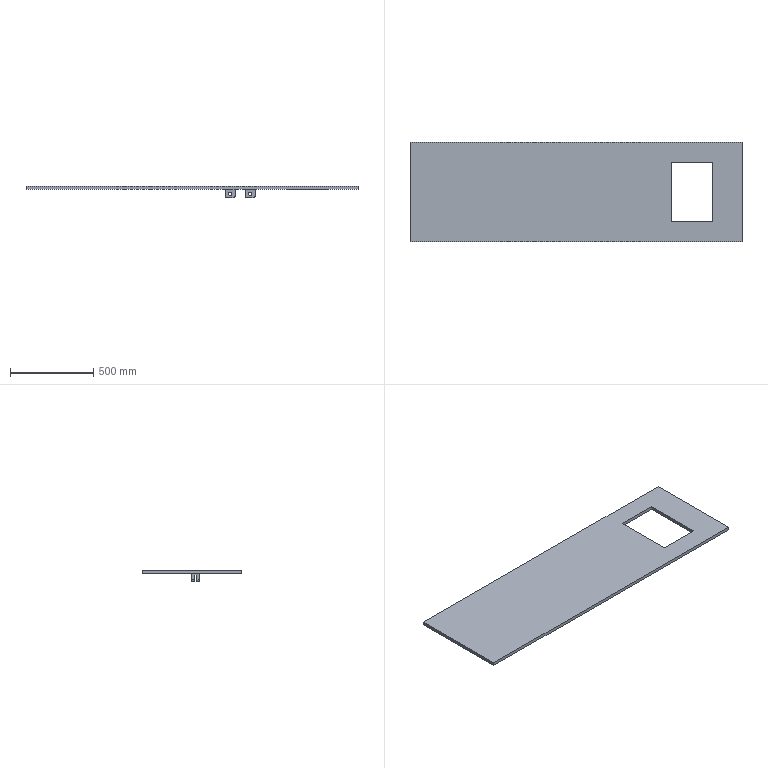Part | SolidWorks | features ICE 3, Cut 1, Extrusion 1, Fillet 1, LPattern 1 | 1 solid | 44 faces | box 2000 x 600 x 71 mm | volume 22419827 mm3 | plane 28 | cylinder 16 | commonest cylinder face diameters 20 x8 24 x8
STEP:
#1=CARTESIAN_POINT('',(220.,2.5,-26.));
#2=VERTEX_POINT('',#1);
#3=CARTESIAN_POINT('',(240.,2.5,-26.));
#4=VERTEX_POINT('',#3);
#5=CARTESIAN_POINT('',(230.,2.5,-26.));
#6=DIRECTION('',(0.,-1.,0.));
#7=DIRECTION('',(1.,0.,0.));
#8=AXIS2_PLACEMENT_3D('',#5,#6,#7);
#9=CIRCLE('',#8,10.);
#10=EDGE_CURVE('',#2,#4,#9,.T.);
#11=ORIENTED_EDGE('',*,*,#10,.F.);
#12=CARTESIAN_POINT('',(220.,-17.5,-26.));
#13=VERTEX_POINT('',#12);
#14=CARTESIAN_POINT('',(220.,300.,-26.));
#15=DIRECTION('',(0.,-1.,0.));
#16=VECTOR('',#15,1000.);
#17=LINE('',#14,#16);
#18=EDGE_CURVE('',#2,#13,#17,.T.);
#19=ORIENTED_EDGE('',*,*,#18,.T.);
#20=CARTESIAN_POINT('',(240.,-17.5,-26.));
#21=VERTEX_POINT('',#20);
#22=CARTESIAN_POINT('',(230.,-17.5,-26.));
#23=DIRECTION('',(0.,1.,0.));
#24=DIRECTION('',(0.,0.,1.));
#25=AXIS2_PLACEMENT_3D('',#22,#23,#24);
#26=CIRCLE('',#25,10.);
#27=EDGE_CURVE('',#21,#13,#26,.T.);
#28=ORIENTED_EDGE('',*,*,#27,.F.);
#29=CARTESIAN_POINT('',(240.,300.,-26.));
#30=DIRECTION('',(0.,-1.,0.));
#31=VECTOR('',#30,1000.);
#32=LINE('',#29,#31);
#33=EDGE_CURVE('',#4,#21,#32,.T.);
#34=ORIENTED_EDGE('',*,*,#33,.F.);
#35=EDGE_LOOP('',(#11,#19,#28,#34));
#36=FACE_OUTER_BOUND('',#35,.T.);
#37=CARTESIAN_POINT('',(230.,300.,-26.));
#38=DIRECTION('',(0.,-1.,0.));
#39=DIRECTION('',(1.,0.,0.));
#40=AXIS2_PLACEMENT_3D('',#37,#38,#39);
#41=CYLINDRICAL_SURFACE('',#40,10.);
#42=ADVANCED_FACE('',(#36),#41,.F.);
#43=CARTESIAN_POINT('',(220.,-29.5,-26.));
#44=VERTEX_POINT('',#43);
#45=CARTESIAN_POINT('',(240.,-29.5,-26.));
#46=VERTEX_POINT('',#45);
#47=CARTESIAN_POINT('',(230.,-29.5,-26.));
#48=DIRECTION('',(0.,-1.,0.));
#49=DIRECTION('',(0.,0.,-1.));
#50=AXIS2_PLACEMENT_3D('',#47,#48,#49);
#51=CIRCLE('',#50,10.);
#52=EDGE_CURVE('',#44,#46,#51,.T.);
#53=ORIENTED_EDGE('',*,*,#52,.F.);
#54=CARTESIAN_POINT('',(220.,-47.5,-26.));
#55=VERTEX_POINT('',#54);
#56=CARTESIAN_POINT('',(220.,300.,-26.));
#57=DIRECTION('',(0.,-1.,0.));
#58=VECTOR('',#57,1000.);
#59=LINE('',#56,#58);
#60=EDGE_CURVE('',#44,#55,#59,.T.);
#61=ORIENTED_EDGE('',*,*,#60,.T.);
#62=CARTESIAN_POINT('',(240.,-47.5,-26.));
#63=VERTEX_POINT('',#62);
#64=CARTESIAN_POINT('',(230.,-47.5,-26.));
#65=DIRECTION('',(0.,-1.,0.));
#66=DIRECTION('',(1.,0.,0.));
#67=AXIS2_PLACEMENT_3D('',#64,#65,#66);
#68=CIRCLE('',#67,10.);
#69=EDGE_CURVE('',#55,#63,#68,.T.);
#70=ORIENTED_EDGE('',*,*,#69,.T.);
#71=CARTESIAN_POINT('',(240.,300.,-26.));
#72=DIRECTION('',(0.,-1.,0.));
#73=VECTOR('',#72,1000.);
#74=LINE('',#71,#73);
#75=EDGE_CURVE('',#46,#63,#74,.T.);
#76=ORIENTED_EDGE('',*,*,#75,.F.);
#77=EDGE_LOOP('',(#53,#61,#70,#76));
#78=FACE_OUTER_BOUND('',#77,.T.);
#79=CARTESIAN_POINT('',(230.,300.,-26.));
#80=DIRECTION('',(0.,-1.,0.));
#81=DIRECTION('',(1.,0.,0.));
#82=AXIS2_PLACEMENT_3D('',#79,#80,#81);
#83=CYLINDRICAL_SURFACE('',#82,10.);
#84=ADVANCED_FACE('',(#78),#83,.F.);
#85=CARTESIAN_POINT('',(340.,2.5,-26.));
#86=VERTEX_POINT('',#85);
#87=CARTESIAN_POINT('',(360.,2.5,-26.));
#88=VERTEX_POINT('',#87);
#89=CARTESIAN_POINT('',(350.,2.5,-26.));
#90=DIRECTION('',(0.,-1.,0.));
#91=DIRECTION('',(1.,0.,0.));
#92=AXIS2_PLACEMENT_3D('',#89,#90,#91);
#93=CIRCLE('',#92,10.);
#94=EDGE_CURVE('',#86,#88,#93,.T.);
#95=ORIENTED_EDGE('',*,*,#94,.F.);
#96=CARTESIAN_POINT('',(340.,-17.5,-26.));
#97=VERTEX_POINT('',#96);
#98=CARTESIAN_POINT('',(340.,300.,-26.));
#99=DIRECTION('',(0.,-1.,0.));
#100=VECTOR('',#99,1000.);
#101=LINE('',#98,#100);
#102=EDGE_CURVE('',#86,#97,#101,.T.);
#103=ORIENTED_EDGE('',*,*,#102,.T.);
#104=CARTESIAN_POINT('',(360.,-17.5,-26.));
#105=VERTEX_POINT('',#104);
#106=CARTESIAN_POINT('',(350.,-17.5,-26.));
#107=DIRECTION('',(0.,1.,0.));
#108=DIRECTION('',(0.,0.,1.));
#109=AXIS2_PLACEMENT_3D('',#106,#107,#108);
#110=CIRCLE('',#109,10.);
#111=EDGE_CURVE('',#105,#97,#110,.T.);
#112=ORIENTED_EDGE('',*,*,#111,.F.);
#113=CARTESIAN_POINT('',(360.,300.,-26.));
#114=DIRECTION('',(0.,-1.,0.));
#115=VECTOR('',#114,1000.);
#116=LINE('',#113,#115);
#117=EDGE_CURVE('',#88,#105,#116,.T.);
#118=ORIENTED_EDGE('',*,*,#117,.F.);
#119=EDGE_LOOP('',(#95,#103,#112,#118));
#120=FACE_OUTER_BOUND('',#119,.T.);
#121=CARTESIAN_POINT('',(350.,300.,-26.));
#122=DIRECTION('',(0.,-1.,0.));
#123=DIRECTION('',(1.,0.,0.));
#124=AXIS2_PLACEMENT_3D('',#121,#122,#123);
#125=CYLINDRICAL_SURFACE('',#124,10.);
#126=ADVANCED_FACE('',(#120),#125,.F.);
#127=CARTESIAN_POINT('',(340.,-29.5,-26.));
#128=VERTEX_POINT('',#127);
#129=CARTESIAN_POINT('',(360.,-29.5,-26.));
#130=VERTEX_POINT('',#129);
#131=CARTESIAN_POINT('',(350.,-29.5,-26.));
#132=DIRECTION('',(0.,-1.,0.));
#133=DIRECTION('',(0.,0.,-1.));
#134=AXIS2_PLACEMENT_3D('',#131,#132,#133);
#135=CIRCLE('',#134,10.);
#136=EDGE_CURVE('',#128,#130,#135,.T.);
#137=ORIENTED_EDGE('',*,*,#136,.F.);
#138=CARTESIAN_POINT('',(340.,-47.5,-26.));
#139=VERTEX_POINT('',#138);
#140=CARTESIAN_POINT('',(340.,300.,-26.));
#141=DIRECTION('',(0.,-1.,0.));
#142=VECTOR('',#141,1000.);
#143=LINE('',#140,#142);
#144=EDGE_CURVE('',#128,#139,#143,.T.);
#145=ORIENTED_EDGE('',*,*,#144,.T.);
#146=CARTESIAN_POINT('',(360.,-47.5,-26.));
#147=VERTEX_POINT('',#146);
#148=CARTESIAN_POINT('',(350.,-47.5,-26.));
#149=DIRECTION('',(0.,-1.,0.));
#150=DIRECTION('',(1.,0.,0.));
#151=AXIS2_PLACEMENT_3D('',#148,#149,#150);
#152=CIRCLE('',#151,10.);
#153=EDGE_CURVE('',#139,#147,#152,.T.);
#154=ORIENTED_EDGE('',*,*,#153,.T.);
#155=CARTESIAN_POINT('',(360.,300.,-26.));
#156=DIRECTION('',(0.,-1.,0.));
#157=VECTOR('',#156,1000.);
#158=LINE('',#155,#157);
#159=EDGE_CURVE('',#130,#147,#158,.T.);
#160=ORIENTED_EDGE('',*,*,#159,.F.);
#161=EDGE_LOOP('',(#137,#145,#154,#160));
#162=FACE_OUTER_BOUND('',#161,.T.);
#163=CARTESIAN_POINT('',(350.,300.,-26.));
#164=DIRECTION('',(0.,-1.,0.));
#165=DIRECTION('',(1.,0.,0.));
#166=AXIS2_PLACEMENT_3D('',#163,#164,#165);
#167=CYLINDRICAL_SURFACE('',#166,10.);
#168=ADVANCED_FACE('',(#162),#167,.F.);
#169=CARTESIAN_POINT('',(212.,-17.5,-51.));
#170=VERTEX_POINT('',#169);
#171=CARTESIAN_POINT('',(248.,-17.5,-51.));
#172=VERTEX_POINT('',#171);
#173=CARTESIAN_POINT('',(260.,-17.5,-51.));
#174=DIRECTION('',(1.,0.,0.));
#175=VECTOR('',#174,1000.);
#176=LINE('',#173,#175);
#177=EDGE_CURVE('',#170,#172,#176,.T.);
#178=ORIENTED_EDGE('',*,*,#177,.F.);
#179=CARTESIAN_POINT('',(212.,2.5,-51.));
#180=VERTEX_POINT('',#179);
#181=CARTESIAN_POINT('',(212.,2.5,-51.));
#182=DIRECTION('',(0.,1.,0.));
#183=VECTOR('',#182,1000.);
#184=LINE('',#181,#183);
#185=EDGE_CURVE('',#170,#180,#184,.T.);
#186=ORIENTED_EDGE('',*,*,#185,.T.);
#187=CARTESIAN_POINT('',(248.,2.5,-51.));
#188=VERTEX_POINT('',#187);
#189=CARTESIAN_POINT('',(200.,2.5,-51.));
#190=DIRECTION('',(1.,0.,0.));
#191=VECTOR('',#190,1000.);
#192=LINE('',#189,#191);
#193=EDGE_CURVE('',#180,#188,#192,.T.);
#194=ORIENTED_EDGE('',*,*,#193,.T.);
#195=CARTESIAN_POINT('',(248.,-17.5,-51.));
#196=DIRECTION('',(0.,-1.,0.));
#197=VECTOR('',#196,1000.);
#198=LINE('',#195,#197);
#199=EDGE_CURVE('',#188,#172,#198,.T.);
#200=ORIENTED_EDGE('',*,*,#199,.T.);
#201=EDGE_LOOP('',(#178,#186,#194,#200));
#202=FACE_OUTER_BOUND('',#201,.T.);
#203=CARTESIAN_POINT('',(-120.,0.,-51.));
#204=DIRECTION('',(0.,0.,-1.));
#205=DIRECTION('',(-1.,0.,0.));
#206=AXIS2_PLACEMENT_3D('',#203,#204,#205);
#207=PLANE('',#206);
#208=ADVANCED_FACE('',(#202),#207,.T.);
#209=CARTESIAN_POINT('',(380.,2.5,0.));
#210=VERTEX_POINT('',#209);
#211=CARTESIAN_POINT('',(380.,-47.5,0.));
#212=VERTEX_POINT('',#211);
#213=CARTESIAN_POINT('',(380.,-47.5,0.));
#214=DIRECTION('',(0.,-1.,0.));
#215=VECTOR('',#214,1000.);
#216=LINE('',#213,#215);
#217=EDGE_CURVE('',#210,#212,#216,.T.);
#218=ORIENTED_EDGE('',*,*,#217,.F.);
#219=CARTESIAN_POINT('',(320.,2.5,0.));
#220=VERTEX_POINT('',#219);
#221=CARTESIAN_POINT('',(320.,2.5,0.));
#222=DIRECTION('',(1.,0.,0.));
#223=VECTOR('',#222,1000.);
#224=LINE('',#221,#223);
#225=EDGE_CURVE('',#220,#210,#224,.T.);
#226=ORIENTED_EDGE('',*,*,#225,.F.);
#227=CARTESIAN_POINT('',(320.,-47.5,0.));
#228=VERTEX_POINT('',#227);
#229=CARTESIAN_POINT('',(320.,-47.5,0.));
#230=DIRECTION('',(0.,1.,0.));
#231=VECTOR('',#230,1000.);
#232=LINE('',#229,#231);
#233=EDGE_CURVE('',#228,#220,#232,.T.);
#234=ORIENTED_EDGE('',*,*,#233,.F.);
#235=CARTESIAN_POINT('',(320.,-47.5,0.));
#236=DIRECTION('',(-1.,0.,0.));
#237=VECTOR('',#236,1000.);
#238=LINE('',#235,#237);
#239=EDGE_CURVE('',#212,#228,#238,.T.);
#240=ORIENTED_EDGE('',*,*,#239,.F.);
#241=EDGE_LOOP('',(#218,#226,#234,#240));
#242=FACE_BOUND('',#241,.T.);
#243=CARTESIAN_POINT('',(825.,-180.,0.));
#244=VERTEX_POINT('',#243);
#245=CARTESIAN_POINT('',(575.,-180.,0.));
#246=VERTEX_POINT('',#245);
#247=CARTESIAN_POINT('',(575.,-180.,0.));
#248=DIRECTION('',(-1.,0.,0.));
#249=VECTOR('',#248,1000.);
#250=LINE('',#247,#249);
#251=EDGE_CURVE('',#244,#246,#250,.T.);
#252=ORIENTED_EDGE('',*,*,#251,.F.);
#253=CARTESIAN_POINT('',(825.,180.,0.));
#254=VERTEX_POINT('',#253);
#255=CARTESIAN_POINT('',(825.,-180.,0.));
#256=DIRECTION('',(0.,-1.,0.));
#257=VECTOR('',#256,1000.);
#258=LINE('',#255,#257);
#259=EDGE_CURVE('',#254,#244,#258,.T.);
#260=ORIENTED_EDGE('',*,*,#259,.F.);
#261=CARTESIAN_POINT('',(575.,180.,0.));
#262=VERTEX_POINT('',#261);
#263=CARTESIAN_POINT('',(575.,180.,0.));
#264=DIRECTION('',(1.,0.,0.));
#265=VECTOR('',#264,1000.);
#266=LINE('',#263,#265);
#267=EDGE_CURVE('',#262,#254,#266,.T.);
#268=ORIENTED_EDGE('',*,*,#267,.F.);
#269=CARTESIAN_POINT('',(575.,-180.,0.));
#270=DIRECTION('',(0.,1.,0.));
#271=VECTOR('',#270,1000.);
#272=LINE('',#269,#271);
#273=EDGE_CURVE('',#246,#262,#272,.T.);
#274=ORIENTED_EDGE('',*,*,#273,.F.);
#275=EDGE_LOOP('',(#252,#260,#268,#274));
#276=FACE_BOUND('',#275,.T.);
#277=CARTESIAN_POINT('',(1000.,-300.,0.));
#278=VERTEX_POINT('',#277);
#279=CARTESIAN_POINT('',(1000.,300.,0.));
#280=VERTEX_POINT('',#279);
#281=CARTESIAN_POINT('',(1000.,300.,0.));
#282=DIRECTION('',(0.,1.,0.));
#283=VECTOR('',#282,1000.);
#284=LINE('',#281,#283);
#285=EDGE_CURVE('',#278,#280,#284,.T.);
#286=ORIENTED_EDGE('',*,*,#285,.F.);
#287=CARTESIAN_POINT('',(-1000.,-300.,0.));
#288=VERTEX_POINT('',#287);
#289=CARTESIAN_POINT('',(-1000.,-300.,0.));
#290=DIRECTION('',(1.,0.,0.));
#291=VECTOR('',#290,1000.);
#292=LINE('',#289,#291);
#293=EDGE_CURVE('',#288,#278,#292,.T.);
#294=ORIENTED_EDGE('',*,*,#293,.F.);
#295=CARTESIAN_POINT('',(-1000.,300.,0.));
#296=VERTEX_POINT('',#295);
#297=CARTESIAN_POINT('',(-1000.,300.,0.));
#298=DIRECTION('',(0.,-1.,0.));
#299=VECTOR('',#298,1000.);
#300=LINE('',#297,#299);
#301=EDGE_CURVE('',#296,#288,#300,.T.);
#302=ORIENTED_EDGE('',*,*,#301,.F.);
#303=CARTESIAN_POINT('',(-1000.,300.,0.));
#304=DIRECTION('',(-1.,0.,0.));
#305=VECTOR('',#304,1000.);
#306=LINE('',#303,#305);
#307=EDGE_CURVE('',#280,#296,#306,.T.);
#308=ORIENTED_EDGE('',*,*,#307,.F.);
#309=EDGE_LOOP('',(#286,#294,#302,#308));
#310=FACE_OUTER_BOUND('',#309,.T.);
#311=CARTESIAN_POINT('',(260.,2.5,0.));
#312=VERTEX_POINT('',#311);
#313=CARTESIAN_POINT('',(260.,-47.5,0.));
#314=VERTEX_POINT('',#313);
#315=CARTESIAN_POINT('',(260.,-47.5,0.));
#316=DIRECTION('',(0.,-1.,0.));
#317=VECTOR('',#316,1000.);
#318=LINE('',#315,#317);
#319=EDGE_CURVE('',#312,#314,#318,.T.);
#320=ORIENTED_EDGE('',*,*,#319,.F.);
#321=CARTESIAN_POINT('',(200.,2.5,0.));
#322=VERTEX_POINT('',#321);
#323=CARTESIAN_POINT('',(200.,2.5,0.));
#324=DIRECTION('',(1.,0.,0.));
#325=VECTOR('',#324,1000.);
#326=LINE('',#323,#325);
#327=EDGE_CURVE('',#322,#312,#326,.T.);
#328=ORIENTED_EDGE('',*,*,#327,.F.);
#329=CARTESIAN_POINT('',(200.,-47.5,0.));
#330=VERTEX_POINT('',#329);
#331=CARTESIAN_POINT('',(200.,-47.5,0.));
#332=DIRECTION('',(0.,1.,0.));
#333=VECTOR('',#332,1000.);
#334=LINE('',#331,#333);
#335=EDGE_CURVE('',#330,#322,#334,.T.);
#336=ORIENTED_EDGE('',*,*,#335,.F.);
#337=CARTESIAN_POINT('',(200.,-47.5,0.));
#338=DIRECTION('',(-1.,0.,0.));
#339=VECTOR('',#338,1000.);
#340=LINE('',#337,#339);
#341=EDGE_CURVE('',#314,#330,#340,.T.);
#342=ORIENTED_EDGE('',*,*,#341,.F.);
#343=EDGE_LOOP('',(#320,#328,#336,#342));
#344=FACE_BOUND('',#343,.T.);
#345=CARTESIAN_POINT('',(0.,0.,0.));
#346=DIRECTION('',(0.,0.,1.));
#347=DIRECTION('',(1.,0.,0.));
#348=AXIS2_PLACEMENT_3D('',#345,#346,#347);
#349=PLANE('',#348);
#350=ADVANCED_FACE('',(#242,#276,#310,#344),#349,.F.);
#351=CARTESIAN_POINT('',(332.,-17.5,-51.));
#352=VERTEX_POINT('',#351);
#353=CARTESIAN_POINT('',(368.,-17.5,-51.));
#354=VERTEX_POINT('',#353);
#355=CARTESIAN_POINT('',(380.,-17.5,-51.));
#356=DIRECTION('',(1.,0.,0.));
#357=VECTOR('',#356,1000.);
#358=LINE('',#355,#357);
#359=EDGE_CURVE('',#352,#354,#358,.T.);
#360=ORIENTED_EDGE('',*,*,#359,.F.);
#361=CARTESIAN_POINT('',(332.,2.5,-51.));
#362=VERTEX_POINT('',#361);
#363=CARTESIAN_POINT('',(332.,2.5,-51.));
#364=DIRECTION('',(0.,1.,0.));
#365=VECTOR('',#364,1000.);
#366=LINE('',#363,#365);
#367=EDGE_CURVE('',#352,#362,#366,.T.);
#368=ORIENTED_EDGE('',*,*,#367,.T.);
#369=CARTESIAN_POINT('',(368.,2.5,-51.));
#370=VERTEX_POINT('',#369);
#371=CARTESIAN_POINT('',(320.,2.5,-51.));
#372=DIRECTION('',(1.,0.,0.));
#373=VECTOR('',#372,1000.);
#374=LINE('',#371,#373);
#375=EDGE_CURVE('',#362,#370,#374,.T.);
#376=ORIENTED_EDGE('',*,*,#375,.T.);
#377=CARTESIAN_POINT('',(368.,-17.5,-51.));
#378=DIRECTION('',(0.,-1.,0.));
#379=VECTOR('',#378,1000.);
#380=LINE('',#377,#379);
#381=EDGE_CURVE('',#370,#354,#380,.T.);
#382=ORIENTED_EDGE('',*,*,#381,.T.);
#383=EDGE_LOOP('',(#360,#368,#376,#382));
#384=FACE_OUTER_BOUND('',#383,.T.);
#385=CARTESIAN_POINT('',(0.,0.,-51.));
#386=DIRECTION('',(0.,0.,-1.));
#387=DIRECTION('',(-1.,0.,0.));
#388=AXIS2_PLACEMENT_3D('',#385,#386,#387);
#389=PLANE('',#388);
#390=ADVANCED_FACE('',(#384),#389,.T.);
#391=ORIENTED_EDGE('',*,*,#285,.T.);
#392=CARTESIAN_POINT('',(1000.,300.,20.));
#393=VERTEX_POINT('',#392);
#394=CARTESIAN_POINT('',(1000.,300.,20.));
#395=DIRECTION('',(0.,0.,-1.));
#396=VECTOR('',#395,1000.);
#397=LINE('',#394,#396);
#398=EDGE_CURVE('',#393,#280,#397,.T.);
#399=ORIENTED_EDGE('',*,*,#398,.F.);
#400=CARTESIAN_POINT('',(1000.,-300.,20.));
#401=VERTEX_POINT('',#400);
#402=CARTESIAN_POINT('',(1000.,300.,20.));
#403=DIRECTION('',(0.,1.,0.));
#404=VECTOR('',#403,1000.);
#405=LINE('',#402,#404);
#406=EDGE_CURVE('',#401,#393,#405,.T.);
#407=ORIENTED_EDGE('',*,*,#406,.F.);
#408=CARTESIAN_POINT('',(1000.,-300.,20.));
#409=DIRECTION('',(0.,0.,-1.));
#410=VECTOR('',#409,1000.);
#411=LINE('',#408,#410);
#412=EDGE_CURVE('',#401,#278,#411,.T.);
#413=ORIENTED_EDGE('',*,*,#412,.T.);
#414=EDGE_LOOP('',(#391,#399,#407,#413));
#415=FACE_OUTER_BOUND('',#414,.T.);
#416=CARTESIAN_POINT('',(1000.,300.,20.));
#417=DIRECTION('',(-1.,0.,0.));
#418=DIRECTION('',(0.,-1.,0.));
#419=AXIS2_PLACEMENT_3D('',#416,#417,#418);
#420=PLANE('',#419);
#421=ADVANCED_FACE('',(#415),#420,.F.);
#422=ORIENTED_EDGE('',*,*,#307,.T.);
#423=CARTESIAN_POINT('',(-1000.,300.,20.));
#424=VERTEX_POINT('',#423);
#425=CARTESIAN_POINT('',(-1000.,300.,20.));
#426=DIRECTION('',(0.,0.,-1.));
#427=VECTOR('',#426,1000.);
#428=LINE('',#425,#427);
#429=EDGE_CURVE('',#424,#296,#428,.T.);
#430=ORIENTED_EDGE('',*,*,#429,.F.);
#431=CARTESIAN_POINT('',(-1000.,300.,20.));
#432=DIRECTION('',(-1.,0.,0.));
#433=VECTOR('',#432,1000.);
#434=LINE('',#431,#433);
#435=EDGE_CURVE('',#393,#424,#434,.T.);
#436=ORIENTED_EDGE('',*,*,#435,.F.);
#437=ORIENTED_EDGE('',*,*,#398,.T.);
#438=EDGE_LOOP('',(#422,#430,#436,#437));
#439=FACE_OUTER_BOUND('',#438,.T.);
#440=CARTESIAN_POINT('',(-1000.,300.,20.));
#441=DIRECTION('',(0.,-1.,0.));
#442=DIRECTION('',(0.,0.,-1.));
#443=AXIS2_PLACEMENT_3D('',#440,#441,#442);
#444=PLANE('',#443);
#445=ADVANCED_FACE('',(#439),#444,.F.);
#446=ORIENTED_EDGE('',*,*,#301,.T.);
#447=CARTESIAN_POINT('',(-1000.,-300.,20.));
#448=VERTEX_POINT('',#447);
#449=CARTESIAN_POINT('',(-1000.,-300.,20.));
#450=DIRECTION('',(0.,0.,-1.));
#451=VECTOR('',#450,1000.);
#452=LINE('',#449,#451);
#453=EDGE_CURVE('',#448,#288,#452,.T.);
#454=ORIENTED_EDGE('',*,*,#453,.F.);
#455=CARTESIAN_POINT('',(-1000.,300.,20.));
#456=DIRECTION('',(0.,-1.,0.));
#457=VECTOR('',#456,1000.);
#458=LINE('',#455,#457);
#459=EDGE_CURVE('',#424,#448,#458,.T.);
#460=ORIENTED_EDGE('',*,*,#459,.F.);
#461=ORIENTED_EDGE('',*,*,#429,.T.);
#462=EDGE_LOOP('',(#446,#454,#460,#461));
#463=FACE_OUTER_BOUND('',#462,.T.);
#464=CARTESIAN_POINT('',(-1000.,300.,20.));
#465=DIRECTION('',(1.,0.,0.));
#466=DIRECTION('',(0.,0.,-1.));
#467=AXIS2_PLACEMENT_3D('',#464,#465,#466);
#468=PLANE('',#467);
#469=ADVANCED_FACE('',(#463),#468,.F.);
#470=ORIENTED_EDGE('',*,*,#293,.T.);
#471=ORIENTED_EDGE('',*,*,#412,.F.);
#472=CARTESIAN_POINT('',(-1000.,-300.,20.));
#473=DIRECTION('',(1.,0.,0.));
#474=VECTOR('',#473,1000.);
#475=LINE('',#472,#474);
#476=EDGE_CURVE('',#448,#401,#475,.T.);
#477=ORIENTED_EDGE('',*,*,#476,.F.);
#478=ORIENTED_EDGE('',*,*,#453,.T.);
#479=EDGE_LOOP('',(#470,#471,#477,#478));
#480=FACE_OUTER_BOUND('',#479,.T.);
#481=CARTESIAN_POINT('',(-1000.,-300.,20.));
#482=DIRECTION('',(0.,1.,0.));
#483=DIRECTION('',(0.,0.,1.));
#484=AXIS2_PLACEMENT_3D('',#481,#482,#483);
#485=PLANE('',#484);
#486=ADVANCED_FACE('',(#480),#485,.F.);
#487=CARTESIAN_POINT('',(825.,180.,20.));
#488=VERTEX_POINT('',#487);
#489=CARTESIAN_POINT('',(825.,-180.,20.));
#490=VERTEX_POINT('',#489);
#491=CARTESIAN_POINT('',(825.,-180.,20.));
#492=DIRECTION('',(0.,-1.,0.));
#493=VECTOR('',#492,1000.);
#494=LINE('',#491,#493);
#495=EDGE_CURVE('',#488,#490,#494,.T.);
#496=ORIENTED_EDGE('',*,*,#495,.T.);
#497=CARTESIAN_POINT('',(575.,-180.,20.));
#498=VERTEX_POINT('',#497);
#499=CARTESIAN_POINT('',(575.,-180.,20.));
#500=DIRECTION('',(-1.,0.,0.));
#501=VECTOR('',#500,1000.);
#502=LINE('',#499,#501);
#503=EDGE_CURVE('',#490,#498,#502,.T.);
#504=ORIENTED_EDGE('',*,*,#503,.T.);
#505=CARTESIAN_POINT('',(575.,180.,20.));
#506=VERTEX_POINT('',#505);
#507=CARTESIAN_POINT('',(575.,-180.,20.));
#508=DIRECTION('',(0.,1.,0.));
#509=VECTOR('',#508,1000.);
#510=LINE('',#507,#509);
#511=EDGE_CURVE('',#498,#506,#510,.T.);
#512=ORIENTED_EDGE('',*,*,#511,.T.);
#513=CARTESIAN_POINT('',(575.,180.,20.));
#514=DIRECTION('',(1.,0.,0.));
#515=VECTOR('',#514,1000.);
#516=LINE('',#513,#515);
#517=EDGE_CURVE('',#506,#488,#516,.T.);
#518=ORIENTED_EDGE('',*,*,#517,.T.);
#519=EDGE_LOOP('',(#496,#504,#512,#518));
#520=FACE_BOUND('',#519,.T.);
#521=ORIENTED_EDGE('',*,*,#406,.T.);
#522=ORIENTED_EDGE('',*,*,#435,.T.);
#523=ORIENTED_EDGE('',*,*,#459,.T.);
#524=ORIENTED_EDGE('',*,*,#476,.T.);
#525=EDGE_LOOP('',(#521,#522,#523,#524));
#526=FACE_OUTER_BOUND('',#525,.T.);
#527=CARTESIAN_POINT('',(0.,0.,20.));
#528=DIRECTION('',(0.,0.,1.));
#529=DIRECTION('',(1.,0.,0.));
#530=AXIS2_PLACEMENT_3D('',#527,#528,#529);
#531=PLANE('',#530);
#532=ADVANCED_FACE('',(#520,#526),#531,.T.);
#533=ORIENTED_EDGE('',*,*,#259,.T.);
#534=CARTESIAN_POINT('',(825.,-180.,20.));
#535=DIRECTION('',(0.,0.,-1.));
#536=VECTOR('',#535,1000.);
#537=LINE('',#534,#536);
#538=EDGE_CURVE('',#490,#244,#537,.T.);
#539=ORIENTED_EDGE('',*,*,#538,.F.);
#540=ORIENTED_EDGE('',*,*,#495,.F.);
#541=CARTESIAN_POINT('',(825.,180.,20.));
#542=DIRECTION('',(0.,0.,-1.));
#543=VECTOR('',#542,1000.);
#544=LINE('',#541,#543);
#545=EDGE_CURVE('',#488,#254,#544,.T.);
#546=ORIENTED_EDGE('',*,*,#545,.T.);
#547=EDGE_LOOP('',(#533,#539,#540,#546));
#548=FACE_OUTER_BOUND('',#547,.T.);
#549=CARTESIAN_POINT('',(825.,-180.,20.));
#550=DIRECTION('',(1.,0.,0.));
#551=DIRECTION('',(0.,0.,-1.));
#552=AXIS2_PLACEMENT_3D('',#549,#550,#551);
#553=PLANE('',#552);
#554=ADVANCED_FACE('',(#548),#553,.F.);
#555=ORIENTED_EDGE('',*,*,#267,.T.);
#556=ORIENTED_EDGE('',*,*,#545,.F.);
#557=ORIENTED_EDGE('',*,*,#517,.F.);
#558=CARTESIAN_POINT('',(575.,180.,20.));
#559=DIRECTION('',(0.,0.,-1.));
#560=VECTOR('',#559,1000.);
#561=LINE('',#558,#560);
#562=EDGE_CURVE('',#506,#262,#561,.T.);
#563=ORIENTED_EDGE('',*,*,#562,.T.);
#564=EDGE_LOOP('',(#555,#556,#557,#563));
#565=FACE_OUTER_BOUND('',#564,.T.);
#566=CARTESIAN_POINT('',(575.,180.,20.));
#567=DIRECTION('',(0.,1.,0.));
#568=DIRECTION('',(-1.,0.,0.));
#569=AXIS2_PLACEMENT_3D('',#566,#567,#568);
#570=PLANE('',#569);
#571=ADVANCED_FACE('',(#565),#570,.F.);
#572=ORIENTED_EDGE('',*,*,#273,.T.);
#573=ORIENTED_EDGE('',*,*,#562,.F.);
#574=ORIENTED_EDGE('',*,*,#511,.F.);
#575=CARTESIAN_POINT('',(575.,-180.,20.));
#576=DIRECTION('',(0.,0.,-1.));
#577=VECTOR('',#576,1000.);
#578=LINE('',#575,#577);
#579=EDGE_CURVE('',#498,#246,#578,.T.);
#580=ORIENTED_EDGE('',*,*,#579,.T.);
#581=EDGE_LOOP('',(#572,#573,#574,#580));
#582=FACE_OUTER_BOUND('',#581,.T.);
#583=CARTESIAN_POINT('',(575.,-180.,20.));
#584=DIRECTION('',(-1.,0.,0.));
#585=DIRECTION('',(0.,0.,1.));
#586=AXIS2_PLACEMENT_3D('',#583,#584,#585);
#587=PLANE('',#586);
#588=ADVANCED_FACE('',(#582),#587,.F.);
#589=ORIENTED_EDGE('',*,*,#251,.T.);
#590=ORIENTED_EDGE('',*,*,#579,.F.);
#591=ORIENTED_EDGE('',*,*,#503,.F.);
#592=ORIENTED_EDGE('',*,*,#538,.T.);
#593=EDGE_LOOP('',(#589,#590,#591,#592));
#594=FACE_OUTER_BOUND('',#593,.T.);
#595=CARTESIAN_POINT('',(575.,-180.,20.));
#596=DIRECTION('',(0.,-1.,0.));
#597=DIRECTION('',(1.,0.,0.));
#598=AXIS2_PLACEMENT_3D('',#595,#596,#597);
#599=PLANE('',#598);
#600=ADVANCED_FACE('',(#594),#599,.F.);
#601=CARTESIAN_POINT('',(380.,-17.5,-11.));
#602=VERTEX_POINT('',#601);
#603=CARTESIAN_POINT('',(380.,-17.5,-39.));
#604=VERTEX_POINT('',#603);
#605=CARTESIAN_POINT('',(380.,-17.5,-11.));
#606=DIRECTION('',(0.,0.,-1.));
#607=VECTOR('',#606,1000.);
#608=LINE('',#605,#607);
#609=EDGE_CURVE('',#602,#604,#608,.T.);
#610=ORIENTED_EDGE('',*,*,#609,.T.);
#611=CARTESIAN_POINT('',(380.,2.5,-39.));
#612=VERTEX_POINT('',#611);
#613=CARTESIAN_POINT('',(380.,2.5,-39.));
#614=DIRECTION('',(0.,1.,0.));
#615=VECTOR('',#614,1000.);
#616=LINE('',#613,#615);
#617=EDGE_CURVE('',#604,#612,#616,.T.);
#618=ORIENTED_EDGE('',*,*,#617,.T.);
#619=CARTESIAN_POINT('',(380.,2.5,-51.));
#620=DIRECTION('',(0.,0.,1.));
#621=VECTOR('',#620,1000.);
#622=LINE('',#619,#621);
#623=EDGE_CURVE('',#612,#210,#622,.T.);
#624=ORIENTED_EDGE('',*,*,#623,.T.);
#625=ORIENTED_EDGE('',*,*,#217,.T.);
#626=CARTESIAN_POINT('',(380.,-47.5,-39.));
#627=VERTEX_POINT('',#626);
#628=CARTESIAN_POINT('',(380.,-47.5,-51.));
#629=DIRECTION('',(0.,0.,1.));
#630=VECTOR('',#629,1000.);
#631=LINE('',#628,#630);
#632=EDGE_CURVE('',#627,#212,#631,.T.);
#633=ORIENTED_EDGE('',*,*,#632,.F.);
#634=CARTESIAN_POINT('',(380.,-29.5,-39.));
#635=VERTEX_POINT('',#634);
#636=CARTESIAN_POINT('',(380.,-29.5,-39.));
#637=DIRECTION('',(0.,1.,0.));
#638=VECTOR('',#637,1000.);
#639=LINE('',#636,#638);
#640=EDGE_CURVE('',#627,#635,#639,.T.);
#641=ORIENTED_EDGE('',*,*,#640,.T.);
#642=CARTESIAN_POINT('',(380.,-29.5,-11.));
#643=VERTEX_POINT('',#642);
#644=CARTESIAN_POINT('',(380.,-29.5,-11.));
#645=DIRECTION('',(0.,0.,-1.));
#646=VECTOR('',#645,1000.);
#647=LINE('',#644,#646);
#648=EDGE_CURVE('',#643,#635,#647,.T.);
#649=ORIENTED_EDGE('',*,*,#648,.F.);
#650=CARTESIAN_POINT('',(380.,-17.5,-11.));
#651=DIRECTION('',(0.,-1.,0.));
#652=VECTOR('',#651,1000.);
#653=LINE('',#650,#652);
#654=EDGE_CURVE('',#602,#643,#653,.T.);
#655=ORIENTED_EDGE('',*,*,#654,.F.);
#656=EDGE_LOOP('',(#610,#618,#624,#625,#633,#641,#649,#655));
#657=FACE_OUTER_BOUND('',#656,.T.);
#658=CARTESIAN_POINT('',(380.,-47.5,-51.));
#659=DIRECTION('',(-1.,0.,0.));
#660=DIRECTION('',(0.,0.,1.));
#661=AXIS2_PLACEMENT_3D('',#658,#659,#660);
#662=PLANE('',#661);
#663=ADVANCED_FACE('',(#657),#662,.F.);
#664=CARTESIAN_POINT('',(350.,-47.5,-26.));
#665=DIRECTION('',(0.,-1.,0.));
#666=DIRECTION('',(1.,0.,0.));
#667=AXIS2_PLACEMENT_3D('',#664,#665,#666);
#668=CIRCLE('',#667,10.);
#669=EDGE_CURVE('',#147,#139,#668,.T.);
#670=ORIENTED_EDGE('',*,*,#669,.F.);
#671=ORIENTED_EDGE('',*,*,#153,.F.);
#672=EDGE_LOOP('',(#670,#671));
#673=FACE_BOUND('',#672,.T.);
#674=CARTESIAN_POINT('',(320.,-47.5,-39.));
#675=VERTEX_POINT('',#674);
#676=CARTESIAN_POINT('',(320.,-47.5,-51.));
#677=DIRECTION('',(0.,0.,1.));
#678=VECTOR('',#677,1000.);
#679=LINE('',#676,#678);
#680=EDGE_CURVE('',#675,#228,#679,.T.);
#681=ORIENTED_EDGE('',*,*,#680,.F.);
#682=CARTESIAN_POINT('',(332.,-47.5,-51.));
#683=VERTEX_POINT('',#682);
#684=CARTESIAN_POINT('',(332.,-47.5,-39.));
#685=DIRECTION('',(0.,-1.,0.));
#686=DIRECTION('',(-1.,0.,0.));
#687=AXIS2_PLACEMENT_3D('',#684,#685,#686);
#688=CIRCLE('',#687,12.);
#689=EDGE_CURVE('',#675,#683,#688,.T.);
#690=ORIENTED_EDGE('',*,*,#689,.T.);
#691=CARTESIAN_POINT('',(368.,-47.5,-51.));
#692=VERTEX_POINT('',#691);
#693=CARTESIAN_POINT('',(320.,-47.5,-51.));
#694=DIRECTION('',(-1.,0.,0.));
#695=VECTOR('',#694,1000.);
#696=LINE('',#693,#695);
#697=EDGE_CURVE('',#692,#683,#696,.T.);
#698=ORIENTED_EDGE('',*,*,#697,.F.);
#699=CARTESIAN_POINT('',(368.,-47.5,-39.));
#700=DIRECTION('',(0.,-1.,0.));
#701=DIRECTION('',(-1.,0.,0.));
#702=AXIS2_PLACEMENT_3D('',#699,#700,#701);
#703=CIRCLE('',#702,12.);
#704=EDGE_CURVE('',#692,#627,#703,.T.);
#705=ORIENTED_EDGE('',*,*,#704,.T.);
#706=ORIENTED_EDGE('',*,*,#632,.T.);
#707=ORIENTED_EDGE('',*,*,#239,.T.);
#708=EDGE_LOOP('',(#681,#690,#698,#705,#706,#707));
#709=FACE_OUTER_BOUND('',#708,.T.);
#710=CARTESIAN_POINT('',(320.,-47.5,-51.));
#711=DIRECTION('',(0.,1.,0.));
#712=DIRECTION('',(-1.,0.,0.));
#713=AXIS2_PLACEMENT_3D('',#710,#711,#712);
#714=PLANE('',#713);
#715=ADVANCED_FACE('',(#673,#709),#714,.F.);
#716=CARTESIAN_POINT('',(320.,-29.5,-11.));
#717=VERTEX_POINT('',#716);
#718=CARTESIAN_POINT('',(320.,-29.5,-39.));
#719=VERTEX_POINT('',#718);
#720=CARTESIAN_POINT('',(320.,-29.5,-11.));
#721=DIRECTION('',(0.,0.,-1.));
#722=VECTOR('',#721,1000.);
#723=LINE('',#720,#722);
#724=EDGE_CURVE('',#717,#719,#723,.T.);
#725=ORIENTED_EDGE('',*,*,#724,.T.);
#726=CARTESIAN_POINT('',(320.,-47.5,-39.));
#727=DIRECTION('',(0.,-1.,0.));
#728=VECTOR('',#727,1000.);
#729=LINE('',#726,#728);
#730=EDGE_CURVE('',#719,#675,#729,.T.);
#731=ORIENTED_EDGE('',*,*,#730,.T.);
#732=ORIENTED_EDGE('',*,*,#680,.T.);
#733=ORIENTED_EDGE('',*,*,#233,.T.);
#734=CARTESIAN_POINT('',(320.,2.5,-39.));
#735=VERTEX_POINT('',#734);
#736=CARTESIAN_POINT('',(320.,2.5,-51.));
#737=DIRECTION('',(0.,0.,1.));
#738=VECTOR('',#737,1000.);
#739=LINE('',#736,#738);
#740=EDGE_CURVE('',#735,#220,#739,.T.);
#741=ORIENTED_EDGE('',*,*,#740,.F.);
#742=CARTESIAN_POINT('',(320.,-17.5,-39.));
#743=VERTEX_POINT('',#742);
#744=CARTESIAN_POINT('',(320.,-17.5,-39.));
#745=DIRECTION('',(0.,-1.,0.));
#746=VECTOR('',#745,1000.);
#747=LINE('',#744,#746);
#748=EDGE_CURVE('',#735,#743,#747,.T.);
#749=ORIENTED_EDGE('',*,*,#748,.T.);
#750=CARTESIAN_POINT('',(320.,-17.5,-11.));
#751=VERTEX_POINT('',#750);
#752=CARTESIAN_POINT('',(320.,-17.5,-11.));
#753=DIRECTION('',(0.,0.,-1.));
#754=VECTOR('',#753,1000.);
#755=LINE('',#752,#754);
#756=EDGE_CURVE('',#751,#743,#755,.T.);
#757=ORIENTED_EDGE('',*,*,#756,.F.);
#758=CARTESIAN_POINT('',(320.,-17.5,-11.));
#759=DIRECTION('',(0.,1.,0.));
#760=VECTOR('',#759,1000.);
#761=LINE('',#758,#760);
#762=EDGE_CURVE('',#717,#751,#761,.T.);
#763=ORIENTED_EDGE('',*,*,#762,.F.);
#764=EDGE_LOOP('',(#725,#731,#732,#733,#741,#749,#757,#763));
#765=FACE_OUTER_BOUND('',#764,.T.);
#766=CARTESIAN_POINT('',(320.,-47.5,-51.));
#767=DIRECTION('',(1.,0.,0.));
#768=DIRECTION('',(0.,0.,-1.));
#769=AXIS2_PLACEMENT_3D('',#766,#767,#768);
#770=PLANE('',#769);
#771=ADVANCED_FACE('',(#765),#770,.F.);
#772=CARTESIAN_POINT('',(350.,2.5,-26.));
#773=DIRECTION('',(0.,-1.,0.));
#774=DIRECTION('',(1.,0.,0.));
#775=AXIS2_PLACEMENT_3D('',#772,#773,#774);
#776=CIRCLE('',#775,10.);
#777=EDGE_CURVE('',#88,#86,#776,.T.);
#778=ORIENTED_EDGE('',*,*,#777,.T.);
#779=ORIENTED_EDGE('',*,*,#94,.T.);
#780=EDGE_LOOP('',(#778,#779));
#781=FACE_BOUND('',#780,.T.);
#782=ORIENTED_EDGE('',*,*,#375,.F.);
#783=CARTESIAN_POINT('',(332.,2.5,-39.));
#784=DIRECTION('',(0.,1.,0.));
#785=DIRECTION('',(1.,0.,0.));
#786=AXIS2_PLACEMENT_3D('',#783,#784,#785);
#787=CIRCLE('',#786,12.);
#788=EDGE_CURVE('',#362,#735,#787,.T.);
#789=ORIENTED_EDGE('',*,*,#788,.T.);
#790=ORIENTED_EDGE('',*,*,#740,.T.);
#791=ORIENTED_EDGE('',*,*,#225,.T.);
#792=ORIENTED_EDGE('',*,*,#623,.F.);
#793=CARTESIAN_POINT('',(368.,2.5,-39.));
#794=DIRECTION('',(0.,1.,0.));
#795=DIRECTION('',(1.,0.,0.));
#796=AXIS2_PLACEMENT_3D('',#793,#794,#795);
#797=CIRCLE('',#796,12.);
#798=EDGE_CURVE('',#612,#370,#797,.T.);
#799=ORIENTED_EDGE('',*,*,#798,.T.);
#800=EDGE_LOOP('',(#782,#789,#790,#791,#792,#799));
#801=FACE_OUTER_BOUND('',#800,.T.);
#802=CARTESIAN_POINT('',(320.,2.5,-51.));
#803=DIRECTION('',(0.,-1.,0.));
#804=DIRECTION('',(1.,0.,0.));
#805=AXIS2_PLACEMENT_3D('',#802,#803,#804);
#806=PLANE('',#805);
#807=ADVANCED_FACE('',(#781,#801),#806,.F.);
#808=ORIENTED_EDGE('',*,*,#697,.T.);
#809=CARTESIAN_POINT('',(332.,-29.5,-51.));
#810=VERTEX_POINT('',#809);
#811=CARTESIAN_POINT('',(332.,-29.5,-51.));
#812=DIRECTION('',(0.,1.,0.));
#813=VECTOR('',#812,1000.);
#814=LINE('',#811,#813);
#815=EDGE_CURVE('',#683,#810,#814,.T.);
#816=ORIENTED_EDGE('',*,*,#815,.T.);
#817=CARTESIAN_POINT('',(368.,-29.5,-51.));
#818=VERTEX_POINT('',#817);
#819=CARTESIAN_POINT('',(380.,-29.5,-51.));
#820=DIRECTION('',(-1.,0.,0.));
#821=VECTOR('',#820,1000.);
#822=LINE('',#819,#821);
#823=EDGE_CURVE('',#818,#810,#822,.T.);
#824=ORIENTED_EDGE('',*,*,#823,.F.);
#825=CARTESIAN_POINT('',(368.,-47.5,-51.));
#826=DIRECTION('',(0.,-1.,0.));
#827=VECTOR('',#826,1000.);
#828=LINE('',#825,#827);
#829=EDGE_CURVE('',#818,#692,#828,.T.);
#830=ORIENTED_EDGE('',*,*,#829,.T.);
#831=EDGE_LOOP('',(#808,#816,#824,#830));
#832=FACE_OUTER_BOUND('',#831,.T.);
#833=CARTESIAN_POINT('',(0.,0.,-51.));
#834=DIRECTION('',(0.,0.,-1.));
#835=DIRECTION('',(-1.,0.,0.));
#836=AXIS2_PLACEMENT_3D('',#833,#834,#835);
#837=PLANE('',#836);
#838=ADVANCED_FACE('',(#832),#837,.T.);
#839=ORIENTED_EDGE('',*,*,#111,.T.);
#840=CARTESIAN_POINT('',(350.,-17.5,-26.));
#841=DIRECTION('',(0.,1.,0.));
#842=DIRECTION('',(0.,0.,1.));
#843=AXIS2_PLACEMENT_3D('',#840,#841,#842);
#844=CIRCLE('',#843,10.);
#845=EDGE_CURVE('',#97,#105,#844,.T.);
#846=ORIENTED_EDGE('',*,*,#845,.T.);
#847=EDGE_LOOP('',(#839,#846));
#848=FACE_BOUND('',#847,.T.);
#849=ORIENTED_EDGE('',*,*,#756,.T.);
#850=CARTESIAN_POINT('',(332.,-17.5,-39.));
#851=DIRECTION('',(0.,-1.,0.));
#852=DIRECTION('',(0.,0.,1.));
#853=AXIS2_PLACEMENT_3D('',#850,#851,#852);
#854=CIRCLE('',#853,12.);
#855=EDGE_CURVE('',#743,#352,#854,.T.);
#856=ORIENTED_EDGE('',*,*,#855,.T.);
#857=ORIENTED_EDGE('',*,*,#359,.T.);
#858=CARTESIAN_POINT('',(368.,-17.5,-39.));
#859=DIRECTION('',(0.,-1.,0.));
#860=DIRECTION('',(0.,0.,1.));
#861=AXIS2_PLACEMENT_3D('',#858,#859,#860);
#862=CIRCLE('',#861,12.);
#863=EDGE_CURVE('',#354,#604,#862,.T.);
#864=ORIENTED_EDGE('',*,*,#863,.T.);
#865=ORIENTED_EDGE('',*,*,#609,.F.);
#866=CARTESIAN_POINT('',(380.,-17.5,-11.));
#867=DIRECTION('',(1.,0.,0.));
#868=VECTOR('',#867,1000.);
#869=LINE('',#866,#868);
#870=EDGE_CURVE('',#751,#602,#869,.T.);
#871=ORIENTED_EDGE('',*,*,#870,.F.);
#872=EDGE_LOOP('',(#849,#856,#857,#864,#865,#871));
#873=FACE_OUTER_BOUND('',#872,.T.);
#874=CARTESIAN_POINT('',(380.,-17.5,-11.));
#875=DIRECTION('',(0.,1.,0.));
#876=DIRECTION('',(0.,0.,1.));
#877=AXIS2_PLACEMENT_3D('',#874,#875,#876);
#878=PLANE('',#877);
#879=ADVANCED_FACE('',(#848,#873),#878,.F.);
#880=CARTESIAN_POINT('',(350.,-29.5,-26.));
#881=DIRECTION('',(0.,-1.,0.));
#882=DIRECTION('',(0.,0.,-1.));
#883=AXIS2_PLACEMENT_3D('',#880,#881,#882);
#884=CIRCLE('',#883,10.);
#885=EDGE_CURVE('',#130,#128,#884,.T.);
#886=ORIENTED_EDGE('',*,*,#885,.T.);
#887=ORIENTED_EDGE('',*,*,#136,.T.);
#888=EDGE_LOOP('',(#886,#887));
#889=FACE_BOUND('',#888,.T.);
#890=ORIENTED_EDGE('',*,*,#823,.T.);
#891=CARTESIAN_POINT('',(332.,-29.5,-39.));
#892=DIRECTION('',(0.,1.,0.));
#893=DIRECTION('',(0.,0.,-1.));
#894=AXIS2_PLACEMENT_3D('',#891,#892,#893);
#895=CIRCLE('',#894,12.);
#896=EDGE_CURVE('',#810,#719,#895,.T.);
#897=ORIENTED_EDGE('',*,*,#896,.T.);
#898=ORIENTED_EDGE('',*,*,#724,.F.);
#899=CARTESIAN_POINT('',(380.,-29.5,-11.));
#900=DIRECTION('',(-1.,0.,0.));
#901=VECTOR('',#900,1000.);
#902=LINE('',#899,#901);
#903=EDGE_CURVE('',#643,#717,#902,.T.);
#904=ORIENTED_EDGE('',*,*,#903,.F.);
#905=ORIENTED_EDGE('',*,*,#648,.T.);
#906=CARTESIAN_POINT('',(368.,-29.5,-39.));
#907=DIRECTION('',(0.,1.,0.));
#908=DIRECTION('',(0.,0.,-1.));
#909=AXIS2_PLACEMENT_3D('',#906,#907,#908);
#910=CIRCLE('',#909,12.);
#911=EDGE_CURVE('',#635,#818,#910,.T.);
#912=ORIENTED_EDGE('',*,*,#911,.T.);
#913=EDGE_LOOP('',(#890,#897,#898,#904,#905,#912));
#914=FACE_OUTER_BOUND('',#913,.T.);
#915=CARTESIAN_POINT('',(380.,-29.5,-11.));
#916=DIRECTION('',(0.,-1.,0.));
#917=DIRECTION('',(0.,0.,-1.));
#918=AXIS2_PLACEMENT_3D('',#915,#916,#917);
#919=PLANE('',#918);
#920=ADVANCED_FACE('',(#889,#914),#919,.F.);
#921=ORIENTED_EDGE('',*,*,#654,.T.);
#922=ORIENTED_EDGE('',*,*,#903,.T.);
#923=ORIENTED_EDGE('',*,*,#762,.T.);
#924=ORIENTED_EDGE('',*,*,#870,.T.);
#925=EDGE_LOOP('',(#921,#922,#923,#924));
#926=FACE_OUTER_BOUND('',#925,.T.);
#927=CARTESIAN_POINT('',(0.,0.,-11.));
#928=DIRECTION('',(0.,0.,-1.));
#929=DIRECTION('',(-1.,0.,0.));
#930=AXIS2_PLACEMENT_3D('',#927,#928,#929);
#931=PLANE('',#930);
#932=ADVANCED_FACE('',(#926),#931,.T.);
#933=ORIENTED_EDGE('',*,*,#689,.F.);
#934=ORIENTED_EDGE('',*,*,#730,.F.);
#935=ORIENTED_EDGE('',*,*,#896,.F.);
#936=ORIENTED_EDGE('',*,*,#815,.F.);
#937=EDGE_LOOP('',(#933,#934,#935,#936));
#938=FACE_OUTER_BOUND('',#937,.T.);
#939=CARTESIAN_POINT('',(332.,0.,-39.));
#940=DIRECTION('',(0.,-1.,0.));
#941=DIRECTION('',(0.,0.,-1.));
#942=AXIS2_PLACEMENT_3D('',#939,#940,#941);
#943=CYLINDRICAL_SURFACE('',#942,12.);
#944=ADVANCED_FACE('',(#938),#943,.T.);
#945=ORIENTED_EDGE('',*,*,#855,.F.);
#946=ORIENTED_EDGE('',*,*,#748,.F.);
#947=ORIENTED_EDGE('',*,*,#788,.F.);
#948=ORIENTED_EDGE('',*,*,#367,.F.);
#949=EDGE_LOOP('',(#945,#946,#947,#948));
#950=FACE_OUTER_BOUND('',#949,.T.);
#951=CARTESIAN_POINT('',(332.,0.,-39.));
#952=DIRECTION('',(0.,-1.,0.));
#953=DIRECTION('',(0.,0.,-1.));
#954=AXIS2_PLACEMENT_3D('',#951,#952,#953);
#955=CYLINDRICAL_SURFACE('',#954,12.);
#956=ADVANCED_FACE('',(#950),#955,.T.);
#957=ORIENTED_EDGE('',*,*,#798,.F.);
#958=ORIENTED_EDGE('',*,*,#617,.F.);
#959=ORIENTED_EDGE('',*,*,#863,.F.);
#960=ORIENTED_EDGE('',*,*,#381,.F.);
#961=EDGE_LOOP('',(#957,#958,#959,#960));
#962=FACE_OUTER_BOUND('',#961,.T.);
#963=CARTESIAN_POINT('',(368.,0.,-39.));
#964=DIRECTION('',(0.,1.,0.));
#965=DIRECTION('',(0.,0.,1.));
#966=AXIS2_PLACEMENT_3D('',#963,#964,#965);
#967=CYLINDRICAL_SURFACE('',#966,12.);
#968=ADVANCED_FACE('',(#962),#967,.T.);
#969=ORIENTED_EDGE('',*,*,#911,.F.);
#970=ORIENTED_EDGE('',*,*,#640,.F.);
#971=ORIENTED_EDGE('',*,*,#704,.F.);
#972=ORIENTED_EDGE('',*,*,#829,.F.);
#973=EDGE_LOOP('',(#969,#970,#971,#972));
#974=FACE_OUTER_BOUND('',#973,.T.);
#975=CARTESIAN_POINT('',(368.,0.,-39.));
#976=DIRECTION('',(0.,1.,0.));
#977=DIRECTION('',(0.,0.,1.));
#978=AXIS2_PLACEMENT_3D('',#975,#976,#977);
#979=CYLINDRICAL_SURFACE('',#978,12.);
#980=ADVANCED_FACE('',(#974),#979,.T.);
#981=ORIENTED_EDGE('',*,*,#144,.F.);
#982=ORIENTED_EDGE('',*,*,#885,.F.);
#983=ORIENTED_EDGE('',*,*,#159,.T.);
#984=ORIENTED_EDGE('',*,*,#669,.T.);
#985=EDGE_LOOP('',(#981,#982,#983,#984));
#986=FACE_OUTER_BOUND('',#985,.T.);
#987=CARTESIAN_POINT('',(350.,300.,-26.));
#988=DIRECTION('',(0.,-1.,0.));
#989=DIRECTION('',(1.,0.,0.));
#990=AXIS2_PLACEMENT_3D('',#987,#988,#989);
#991=CYLINDRICAL_SURFACE('',#990,10.);
#992=ADVANCED_FACE('',(#986),#991,.F.);
#993=ORIENTED_EDGE('',*,*,#102,.F.);
#994=ORIENTED_EDGE('',*,*,#777,.F.);
#995=ORIENTED_EDGE('',*,*,#117,.T.);
#996=ORIENTED_EDGE('',*,*,#845,.F.);
#997=EDGE_LOOP('',(#993,#994,#995,#996));
#998=FACE_OUTER_BOUND('',#997,.T.);
#999=CARTESIAN_POINT('',(350.,300.,-26.));
#1000=DIRECTION('',(0.,-1.,0.));
#1001=DIRECTION('',(1.,0.,0.));
#1002=AXIS2_PLACEMENT_3D('',#999,#1000,#1001);
#1003=CYLINDRICAL_SURFACE('',#1002,10.);
#1004=ADVANCED_FACE('',(#998),#1003,.F.);
#1005=CARTESIAN_POINT('',(260.,-17.5,-11.));
#1006=VERTEX_POINT('',#1005);
#1007=CARTESIAN_POINT('',(260.,-17.5,-39.));
#1008=VERTEX_POINT('',#1007);
#1009=CARTESIAN_POINT('',(260.,-17.5,-11.));
#1010=DIRECTION('',(0.,0.,-1.));
#1011=VECTOR('',#1010,1000.);
#1012=LINE('',#1009,#1011);
#1013=EDGE_CURVE('',#1006,#1008,#1012,.T.);
#1014=ORIENTED_EDGE('',*,*,#1013,.T.);
#1015=CARTESIAN_POINT('',(260.,2.5,-39.));
#1016=VERTEX_POINT('',#1015);
#1017=CARTESIAN_POINT('',(260.,2.5,-39.));
#1018=DIRECTION('',(0.,1.,0.));
#1019=VECTOR('',#1018,1000.);
#1020=LINE('',#1017,#1019);
#1021=EDGE_CURVE('',#1008,#1016,#1020,.T.);
#1022=ORIENTED_EDGE('',*,*,#1021,.T.);
#1023=CARTESIAN_POINT('',(260.,2.5,-51.));
#1024=DIRECTION('',(0.,0.,1.));
#1025=VECTOR('',#1024,1000.);
#1026=LINE('',#1023,#1025);
#1027=EDGE_CURVE('',#1016,#312,#1026,.T.);
#1028=ORIENTED_EDGE('',*,*,#1027,.T.);
#1029=ORIENTED_EDGE('',*,*,#319,.T.);
#1030=CARTESIAN_POINT('',(260.,-47.5,-39.));
#1031=VERTEX_POINT('',#1030);
#1032=CARTESIAN_POINT('',(260.,-47.5,-51.));
#1033=DIRECTION('',(0.,0.,1.));
#1034=VECTOR('',#1033,1000.);
#1035=LINE('',#1032,#1034);
#1036=EDGE_CURVE('',#1031,#314,#1035,.T.);
#1037=ORIENTED_EDGE('',*,*,#1036,.F.);
#1038=CARTESIAN_POINT('',(260.,-29.5,-39.));
#1039=VERTEX_POINT('',#1038);
#1040=CARTESIAN_POINT('',(260.,-29.5,-39.));
#1041=DIRECTION('',(0.,1.,0.));
#1042=VECTOR('',#1041,1000.);
#1043=LINE('',#1040,#1042);
#1044=EDGE_CURVE('',#1031,#1039,#1043,.T.);
#1045=ORIENTED_EDGE('',*,*,#1044,.T.);
#1046=CARTESIAN_POINT('',(260.,-29.5,-11.));
#1047=VERTEX_POINT('',#1046);
#1048=CARTESIAN_POINT('',(260.,-29.5,-11.));
#1049=DIRECTION('',(0.,0.,-1.));
#1050=VECTOR('',#1049,1000.);
#1051=LINE('',#1048,#1050);
#1052=EDGE_CURVE('',#1047,#1039,#1051,.T.);
#1053=ORIENTED_EDGE('',*,*,#1052,.F.);
#1054=CARTESIAN_POINT('',(260.,-17.5,-11.));
#1055=DIRECTION('',(0.,-1.,0.));
#1056=VECTOR('',#1055,1000.);
#1057=LINE('',#1054,#1056);
#1058=EDGE_CURVE('',#1006,#1047,#1057,.T.);
#1059=ORIENTED_EDGE('',*,*,#1058,.F.);
#1060=EDGE_LOOP('',(#1014,#1022,#1028,#1029,#1037,#1045,#1053,#1059));
#1061=FACE_OUTER_BOUND('',#1060,.T.);
#1062=CARTESIAN_POINT('',(260.,-47.5,-51.));
#1063=DIRECTION('',(-1.,0.,0.));
#1064=DIRECTION('',(0.,0.,1.));
#1065=AXIS2_PLACEMENT_3D('',#1062,#1063,#1064);
#1066=PLANE('',#1065);
#1067=ADVANCED_FACE('',(#1061),#1066,.F.);
#1068=CARTESIAN_POINT('',(230.,-47.5,-26.));
#1069=DIRECTION('',(0.,-1.,0.));
#1070=DIRECTION('',(1.,0.,0.));
#1071=AXIS2_PLACEMENT_3D('',#1068,#1069,#1070);
#1072=CIRCLE('',#1071,10.);
#1073=EDGE_CURVE('',#63,#55,#1072,.T.);
#1074=ORIENTED_EDGE('',*,*,#1073,.F.);
#1075=ORIENTED_EDGE('',*,*,#69,.F.);
#1076=EDGE_LOOP('',(#1074,#1075));
#1077=FACE_BOUND('',#1076,.T.);
#1078=CARTESIAN_POINT('',(200.,-47.5,-39.));
#1079=VERTEX_POINT('',#1078);
#1080=CARTESIAN_POINT('',(200.,-47.5,-51.));
#1081=DIRECTION('',(0.,0.,1.));
#1082=VECTOR('',#1081,1000.);
#1083=LINE('',#1080,#1082);
#1084=EDGE_CURVE('',#1079,#330,#1083,.T.);
#1085=ORIENTED_EDGE('',*,*,#1084,.F.);
#1086=CARTESIAN_POINT('',(212.,-47.5,-51.));
#1087=VERTEX_POINT('',#1086);
#1088=CARTESIAN_POINT('',(212.,-47.5,-39.));
#1089=DIRECTION('',(0.,-1.,0.));
#1090=DIRECTION('',(-1.,0.,0.));
#1091=AXIS2_PLACEMENT_3D('',#1088,#1089,#1090);
#1092=CIRCLE('',#1091,12.);
#1093=EDGE_CURVE('',#1079,#1087,#1092,.T.);
#1094=ORIENTED_EDGE('',*,*,#1093,.T.);
#1095=CARTESIAN_POINT('',(248.,-47.5,-51.));
#1096=VERTEX_POINT('',#1095);
#1097=CARTESIAN_POINT('',(200.,-47.5,-51.));
#1098=DIRECTION('',(-1.,0.,0.));
#1099=VECTOR('',#1098,1000.);
#1100=LINE('',#1097,#1099);
#1101=EDGE_CURVE('',#1096,#1087,#1100,.T.);
#1102=ORIENTED_EDGE('',*,*,#1101,.F.);
#1103=CARTESIAN_POINT('',(248.,-47.5,-39.));
#1104=DIRECTION('',(0.,-1.,0.));
#1105=DIRECTION('',(-1.,0.,0.));
#1106=AXIS2_PLACEMENT_3D('',#1103,#1104,#1105);
#1107=CIRCLE('',#1106,12.);
#1108=EDGE_CURVE('',#1096,#1031,#1107,.T.);
#1109=ORIENTED_EDGE('',*,*,#1108,.T.);
#1110=ORIENTED_EDGE('',*,*,#1036,.T.);
#1111=ORIENTED_EDGE('',*,*,#341,.T.);
#1112=EDGE_LOOP('',(#1085,#1094,#1102,#1109,#1110,#1111));
#1113=FACE_OUTER_BOUND('',#1112,.T.);
#1114=CARTESIAN_POINT('',(200.,-47.5,-51.));
#1115=DIRECTION('',(0.,1.,0.));
#1116=DIRECTION('',(-1.,0.,0.));
#1117=AXIS2_PLACEMENT_3D('',#1114,#1115,#1116);
#1118=PLANE('',#1117);
#1119=ADVANCED_FACE('',(#1077,#1113),#1118,.F.);
#1120=CARTESIAN_POINT('',(200.,-29.5,-11.));
#1121=VERTEX_POINT('',#1120);
#1122=CARTESIAN_POINT('',(200.,-29.5,-39.));
#1123=VERTEX_POINT('',#1122);
#1124=CARTESIAN_POINT('',(200.,-29.5,-11.));
#1125=DIRECTION('',(0.,0.,-1.));
#1126=VECTOR('',#1125,1000.);
#1127=LINE('',#1124,#1126);
#1128=EDGE_CURVE('',#1121,#1123,#1127,.T.);
#1129=ORIENTED_EDGE('',*,*,#1128,.T.);
#1130=CARTESIAN_POINT('',(200.,-47.5,-39.));
#1131=DIRECTION('',(0.,-1.,0.));
#1132=VECTOR('',#1131,1000.);
#1133=LINE('',#1130,#1132);
#1134=EDGE_CURVE('',#1123,#1079,#1133,.T.);
#1135=ORIENTED_EDGE('',*,*,#1134,.T.);
#1136=ORIENTED_EDGE('',*,*,#1084,.T.);
#1137=ORIENTED_EDGE('',*,*,#335,.T.);
#1138=CARTESIAN_POINT('',(200.,2.5,-39.));
#1139=VERTEX_POINT('',#1138);
#1140=CARTESIAN_POINT('',(200.,2.5,-51.));
#1141=DIRECTION('',(0.,0.,1.));
#1142=VECTOR('',#1141,1000.);
#1143=LINE('',#1140,#1142);
#1144=EDGE_CURVE('',#1139,#322,#1143,.T.);
#1145=ORIENTED_EDGE('',*,*,#1144,.F.);
#1146=CARTESIAN_POINT('',(200.,-17.5,-39.));
#1147=VERTEX_POINT('',#1146);
#1148=CARTESIAN_POINT('',(200.,-17.5,-39.));
#1149=DIRECTION('',(0.,-1.,0.));
#1150=VECTOR('',#1149,1000.);
#1151=LINE('',#1148,#1150);
#1152=EDGE_CURVE('',#1139,#1147,#1151,.T.);
#1153=ORIENTED_EDGE('',*,*,#1152,.T.);
#1154=CARTESIAN_POINT('',(200.,-17.5,-11.));
#1155=VERTEX_POINT('',#1154);
#1156=CARTESIAN_POINT('',(200.,-17.5,-11.));
#1157=DIRECTION('',(0.,0.,-1.));
#1158=VECTOR('',#1157,1000.);
#1159=LINE('',#1156,#1158);
#1160=EDGE_CURVE('',#1155,#1147,#1159,.T.);
#1161=ORIENTED_EDGE('',*,*,#1160,.F.);
#1162=CARTESIAN_POINT('',(200.,-17.5,-11.));
#1163=DIRECTION('',(0.,1.,0.));
#1164=VECTOR('',#1163,1000.);
#1165=LINE('',#1162,#1164);
#1166=EDGE_CURVE('',#1121,#1155,#1165,.T.);
#1167=ORIENTED_EDGE('',*,*,#1166,.F.);
#1168=EDGE_LOOP('',(#1129,#1135,#1136,#1137,#1145,#1153,#1161,#1167));
#1169=FACE_OUTER_BOUND('',#1168,.T.);
#1170=CARTESIAN_POINT('',(200.,-47.5,-51.));
#1171=DIRECTION('',(1.,0.,0.));
#1172=DIRECTION('',(0.,0.,-1.));
#1173=AXIS2_PLACEMENT_3D('',#1170,#1171,#1172);
#1174=PLANE('',#1173);
#1175=ADVANCED_FACE('',(#1169),#1174,.F.);
#1176=CARTESIAN_POINT('',(230.,2.5,-26.));
#1177=DIRECTION('',(0.,-1.,0.));
#1178=DIRECTION('',(1.,0.,0.));
#1179=AXIS2_PLACEMENT_3D('',#1176,#1177,#1178);
#1180=CIRCLE('',#1179,10.);
#1181=EDGE_CURVE('',#4,#2,#1180,.T.);
#1182=ORIENTED_EDGE('',*,*,#1181,.T.);
#1183=ORIENTED_EDGE('',*,*,#10,.T.);
#1184=EDGE_LOOP('',(#1182,#1183));
#1185=FACE_BOUND('',#1184,.T.);
#1186=ORIENTED_EDGE('',*,*,#193,.F.);
#1187=CARTESIAN_POINT('',(212.,2.5,-39.));
#1188=DIRECTION('',(0.,1.,0.));
#1189=DIRECTION('',(1.,0.,0.));
#1190=AXIS2_PLACEMENT_3D('',#1187,#1188,#1189);
#1191=CIRCLE('',#1190,12.);
#1192=EDGE_CURVE('',#180,#1139,#1191,.T.);
#1193=ORIENTED_EDGE('',*,*,#1192,.T.);
#1194=ORIENTED_EDGE('',*,*,#1144,.T.);
#1195=ORIENTED_EDGE('',*,*,#327,.T.);
#1196=ORIENTED_EDGE('',*,*,#1027,.F.);
#1197=CARTESIAN_POINT('',(248.,2.5,-39.));
#1198=DIRECTION('',(0.,1.,0.));
#1199=DIRECTION('',(1.,0.,0.));
#1200=AXIS2_PLACEMENT_3D('',#1197,#1198,#1199);
#1201=CIRCLE('',#1200,12.);
#1202=EDGE_CURVE('',#1016,#188,#1201,.T.);
#1203=ORIENTED_EDGE('',*,*,#1202,.T.);
#1204=EDGE_LOOP('',(#1186,#1193,#1194,#1195,#1196,#1203));
#1205=FACE_OUTER_BOUND('',#1204,.T.);
#1206=CARTESIAN_POINT('',(200.,2.5,-51.));
#1207=DIRECTION('',(0.,-1.,0.));
#1208=DIRECTION('',(1.,0.,0.));
#1209=AXIS2_PLACEMENT_3D('',#1206,#1207,#1208);
#1210=PLANE('',#1209);
#1211=ADVANCED_FACE('',(#1185,#1205),#1210,.F.);
#1212=ORIENTED_EDGE('',*,*,#1101,.T.);
#1213=CARTESIAN_POINT('',(212.,-29.5,-51.));
#1214=VERTEX_POINT('',#1213);
#1215=CARTESIAN_POINT('',(212.,-29.5,-51.));
#1216=DIRECTION('',(0.,1.,0.));
#1217=VECTOR('',#1216,1000.);
#1218=LINE('',#1215,#1217);
#1219=EDGE_CURVE('',#1087,#1214,#1218,.T.);
#1220=ORIENTED_EDGE('',*,*,#1219,.T.);
#1221=CARTESIAN_POINT('',(248.,-29.5,-51.));
#1222=VERTEX_POINT('',#1221);
#1223=CARTESIAN_POINT('',(260.,-29.5,-51.));
#1224=DIRECTION('',(-1.,0.,0.));
#1225=VECTOR('',#1224,1000.);
#1226=LINE('',#1223,#1225);
#1227=EDGE_CURVE('',#1222,#1214,#1226,.T.);
#1228=ORIENTED_EDGE('',*,*,#1227,.F.);
#1229=CARTESIAN_POINT('',(248.,-47.5,-51.));
#1230=DIRECTION('',(0.,-1.,0.));
#1231=VECTOR('',#1230,1000.);
#1232=LINE('',#1229,#1231);
#1233=EDGE_CURVE('',#1222,#1096,#1232,.T.);
#1234=ORIENTED_EDGE('',*,*,#1233,.T.);
#1235=EDGE_LOOP('',(#1212,#1220,#1228,#1234));
#1236=FACE_OUTER_BOUND('',#1235,.T.);
#1237=CARTESIAN_POINT('',(-120.,0.,-51.));
#1238=DIRECTION('',(0.,0.,-1.));
#1239=DIRECTION('',(-1.,0.,0.));
#1240=AXIS2_PLACEMENT_3D('',#1237,#1238,#1239);
#1241=PLANE('',#1240);
#1242=ADVANCED_FACE('',(#1236),#1241,.T.);
#1243=ORIENTED_EDGE('',*,*,#27,.T.);
#1244=CARTESIAN_POINT('',(230.,-17.5,-26.));
#1245=DIRECTION('',(0.,1.,0.));
#1246=DIRECTION('',(0.,0.,1.));
#1247=AXIS2_PLACEMENT_3D('',#1244,#1245,#1246);
#1248=CIRCLE('',#1247,10.);
#1249=EDGE_CURVE('',#13,#21,#1248,.T.);
#1250=ORIENTED_EDGE('',*,*,#1249,.T.);
#1251=EDGE_LOOP('',(#1243,#1250));
#1252=FACE_BOUND('',#1251,.T.);
#1253=ORIENTED_EDGE('',*,*,#1160,.T.);
#1254=CARTESIAN_POINT('',(212.,-17.5,-39.));
#1255=DIRECTION('',(0.,-1.,0.));
#1256=DIRECTION('',(0.,0.,1.));
#1257=AXIS2_PLACEMENT_3D('',#1254,#1255,#1256);
#1258=CIRCLE('',#1257,12.);
#1259=EDGE_CURVE('',#1147,#170,#1258,.T.);
#1260=ORIENTED_EDGE('',*,*,#1259,.T.);
#1261=ORIENTED_EDGE('',*,*,#177,.T.);
#1262=CARTESIAN_POINT('',(248.,-17.5,-39.));
#1263=DIRECTION('',(0.,-1.,0.));
#1264=DIRECTION('',(0.,0.,1.));
#1265=AXIS2_PLACEMENT_3D('',#1262,#1263,#1264);
#1266=CIRCLE('',#1265,12.);
#1267=EDGE_CURVE('',#172,#1008,#1266,.T.);
#1268=ORIENTED_EDGE('',*,*,#1267,.T.);
#1269=ORIENTED_EDGE('',*,*,#1013,.F.);
#1270=CARTESIAN_POINT('',(260.,-17.5,-11.));
#1271=DIRECTION('',(1.,0.,0.));
#1272=VECTOR('',#1271,1000.);
#1273=LINE('',#1270,#1272);
#1274=EDGE_CURVE('',#1155,#1006,#1273,.T.);
#1275=ORIENTED_EDGE('',*,*,#1274,.F.);
#1276=EDGE_LOOP('',(#1253,#1260,#1261,#1268,#1269,#1275));
#1277=FACE_OUTER_BOUND('',#1276,.T.);
#1278=CARTESIAN_POINT('',(260.,-17.5,-11.));
#1279=DIRECTION('',(0.,1.,0.));
#1280=DIRECTION('',(0.,0.,1.));
#1281=AXIS2_PLACEMENT_3D('',#1278,#1279,#1280);
#1282=PLANE('',#1281);
#1283=ADVANCED_FACE('',(#1252,#1277),#1282,.F.);
#1284=CARTESIAN_POINT('',(230.,-29.5,-26.));
#1285=DIRECTION('',(0.,-1.,0.));
#1286=DIRECTION('',(0.,0.,-1.));
#1287=AXIS2_PLACEMENT_3D('',#1284,#1285,#1286);
#1288=CIRCLE('',#1287,10.);
#1289=EDGE_CURVE('',#46,#44,#1288,.T.);
#1290=ORIENTED_EDGE('',*,*,#1289,.T.);
#1291=ORIENTED_EDGE('',*,*,#52,.T.);
#1292=EDGE_LOOP('',(#1290,#1291));
#1293=FACE_BOUND('',#1292,.T.);
#1294=ORIENTED_EDGE('',*,*,#1227,.T.);
#1295=CARTESIAN_POINT('',(212.,-29.5,-39.));
#1296=DIRECTION('',(0.,1.,0.));
#1297=DIRECTION('',(0.,0.,-1.));
#1298=AXIS2_PLACEMENT_3D('',#1295,#1296,#1297);
#1299=CIRCLE('',#1298,12.);
#1300=EDGE_CURVE('',#1214,#1123,#1299,.T.);
#1301=ORIENTED_EDGE('',*,*,#1300,.T.);
#1302=ORIENTED_EDGE('',*,*,#1128,.F.);
#1303=CARTESIAN_POINT('',(260.,-29.5,-11.));
#1304=DIRECTION('',(-1.,0.,0.));
#1305=VECTOR('',#1304,1000.);
#1306=LINE('',#1303,#1305);
#1307=EDGE_CURVE('',#1047,#1121,#1306,.T.);
#1308=ORIENTED_EDGE('',*,*,#1307,.F.);
#1309=ORIENTED_EDGE('',*,*,#1052,.T.);
#1310=CARTESIAN_POINT('',(248.,-29.5,-39.));
#1311=DIRECTION('',(0.,1.,0.));
#1312=DIRECTION('',(0.,0.,-1.));
#1313=AXIS2_PLACEMENT_3D('',#1310,#1311,#1312);
#1314=CIRCLE('',#1313,12.);
#1315=EDGE_CURVE('',#1039,#1222,#1314,.T.);
#1316=ORIENTED_EDGE('',*,*,#1315,.T.);
#1317=EDGE_LOOP('',(#1294,#1301,#1302,#1308,#1309,#1316));
#1318=FACE_OUTER_BOUND('',#1317,.T.);
#1319=CARTESIAN_POINT('',(260.,-29.5,-11.));
#1320=DIRECTION('',(0.,-1.,0.));
#1321=DIRECTION('',(0.,0.,-1.));
#1322=AXIS2_PLACEMENT_3D('',#1319,#1320,#1321);
#1323=PLANE('',#1322);
#1324=ADVANCED_FACE('',(#1293,#1318),#1323,.F.);
#1325=ORIENTED_EDGE('',*,*,#1058,.T.);
#1326=ORIENTED_EDGE('',*,*,#1307,.T.);
#1327=ORIENTED_EDGE('',*,*,#1166,.T.);
#1328=ORIENTED_EDGE('',*,*,#1274,.T.);
#1329=EDGE_LOOP('',(#1325,#1326,#1327,#1328));
#1330=FACE_OUTER_BOUND('',#1329,.T.);
#1331=CARTESIAN_POINT('',(-120.,0.,-11.));
#1332=DIRECTION('',(0.,0.,-1.));
#1333=DIRECTION('',(-1.,0.,0.));
#1334=AXIS2_PLACEMENT_3D('',#1331,#1332,#1333);
#1335=PLANE('',#1334);
#1336=ADVANCED_FACE('',(#1330),#1335,.T.);
#1337=ORIENTED_EDGE('',*,*,#1093,.F.);
#1338=ORIENTED_EDGE('',*,*,#1134,.F.);
#1339=ORIENTED_EDGE('',*,*,#1300,.F.);
#1340=ORIENTED_EDGE('',*,*,#1219,.F.);
#1341=EDGE_LOOP('',(#1337,#1338,#1339,#1340));
#1342=FACE_OUTER_BOUND('',#1341,.T.);
#1343=CARTESIAN_POINT('',(212.,0.,-39.));
#1344=DIRECTION('',(0.,-1.,0.));
#1345=DIRECTION('',(0.,0.,-1.));
#1346=AXIS2_PLACEMENT_3D('',#1343,#1344,#1345);
#1347=CYLINDRICAL_SURFACE('',#1346,12.);
#1348=ADVANCED_FACE('',(#1342),#1347,.T.);
#1349=ORIENTED_EDGE('',*,*,#1259,.F.);
#1350=ORIENTED_EDGE('',*,*,#1152,.F.);
#1351=ORIENTED_EDGE('',*,*,#1192,.F.);
#1352=ORIENTED_EDGE('',*,*,#185,.F.);
#1353=EDGE_LOOP('',(#1349,#1350,#1351,#1352));
#1354=FACE_OUTER_BOUND('',#1353,.T.);
#1355=CARTESIAN_POINT('',(212.,0.,-39.));
#1356=DIRECTION('',(0.,-1.,0.));
#1357=DIRECTION('',(0.,0.,-1.));
#1358=AXIS2_PLACEMENT_3D('',#1355,#1356,#1357);
#1359=CYLINDRICAL_SURFACE('',#1358,12.);
#1360=ADVANCED_FACE('',(#1354),#1359,.T.);
#1361=ORIENTED_EDGE('',*,*,#1202,.F.);
#1362=ORIENTED_EDGE('',*,*,#1021,.F.);
#1363=ORIENTED_EDGE('',*,*,#1267,.F.);
#1364=ORIENTED_EDGE('',*,*,#199,.F.);
#1365=EDGE_LOOP('',(#1361,#1362,#1363,#1364));
#1366=FACE_OUTER_BOUND('',#1365,.T.);
#1367=CARTESIAN_POINT('',(248.,0.,-39.));
#1368=DIRECTION('',(0.,1.,0.));
#1369=DIRECTION('',(0.,0.,1.));
#1370=AXIS2_PLACEMENT_3D('',#1367,#1368,#1369);
#1371=CYLINDRICAL_SURFACE('',#1370,12.);
#1372=ADVANCED_FACE('',(#1366),#1371,.T.);
#1373=ORIENTED_EDGE('',*,*,#1315,.F.);
#1374=ORIENTED_EDGE('',*,*,#1044,.F.);
#1375=ORIENTED_EDGE('',*,*,#1108,.F.);
#1376=ORIENTED_EDGE('',*,*,#1233,.F.);
#1377=EDGE_LOOP('',(#1373,#1374,#1375,#1376));
#1378=FACE_OUTER_BOUND('',#1377,.T.);
#1379=CARTESIAN_POINT('',(248.,0.,-39.));
#1380=DIRECTION('',(0.,1.,0.));
#1381=DIRECTION('',(0.,0.,1.));
#1382=AXIS2_PLACEMENT_3D('',#1379,#1380,#1381);
#1383=CYLINDRICAL_SURFACE('',#1382,12.);
#1384=ADVANCED_FACE('',(#1378),#1383,.T.);
#1385=ORIENTED_EDGE('',*,*,#60,.F.);
#1386=ORIENTED_EDGE('',*,*,#1289,.F.);
#1387=ORIENTED_EDGE('',*,*,#75,.T.);
#1388=ORIENTED_EDGE('',*,*,#1073,.T.);
#1389=EDGE_LOOP('',(#1385,#1386,#1387,#1388));
#1390=FACE_OUTER_BOUND('',#1389,.T.);
#1391=CARTESIAN_POINT('',(230.,300.,-26.));
#1392=DIRECTION('',(0.,-1.,0.));
#1393=DIRECTION('',(1.,0.,0.));
#1394=AXIS2_PLACEMENT_3D('',#1391,#1392,#1393);
#1395=CYLINDRICAL_SURFACE('',#1394,10.);
#1396=ADVANCED_FACE('',(#1390),#1395,.F.);
#1397=ORIENTED_EDGE('',*,*,#18,.F.);
#1398=ORIENTED_EDGE('',*,*,#1181,.F.);
#1399=ORIENTED_EDGE('',*,*,#33,.T.);
#1400=ORIENTED_EDGE('',*,*,#1249,.F.);
#1401=EDGE_LOOP('',(#1397,#1398,#1399,#1400));
#1402=FACE_OUTER_BOUND('',#1401,.T.);
#1403=CARTESIAN_POINT('',(230.,300.,-26.));
#1404=DIRECTION('',(0.,-1.,0.));
#1405=DIRECTION('',(1.,0.,0.));
#1406=AXIS2_PLACEMENT_3D('',#1403,#1404,#1405);
#1407=CYLINDRICAL_SURFACE('',#1406,10.);
#1408=ADVANCED_FACE('',(#1402),#1407,.F.);
#1409=CLOSED_SHELL('',(#42,#84,#126,#168,#208,#350,#390,#421,#445,#469,#486,#532,#554,#571,#588,#600,#663,#715,#771,#807,#838,#879,#920,#932,#944,#956,#968,#980,#992,#1004,#1067,#1119,#1175,#1211,#1242,#1283,#1324,#1336,#1348,#1360,#1372,#1384,#1396,#1408));
#1410=MANIFOLD_SOLID_BREP('',#1409);
#1411=CARTESIAN_POINT('',(0.,0.,0.));
#1412=DIRECTION('',(0.,0.,1.));
#1413=DIRECTION('',(1.,0.,0.));
#1414=AXIS2_PLACEMENT_3D('',#1411,#1412,#1413);
#1415=(LENGTH_UNIT()NAMED_UNIT(*)SI_UNIT(.MILLI.,.METRE.));
#1416=UNCERTAINTY_MEASURE_WITH_UNIT(LENGTH_MEASURE(0.00001),#1415,'','');
#1417=(NAMED_UNIT(*)PLANE_ANGLE_UNIT()SI_UNIT($,.RADIAN.));
#1418=(NAMED_UNIT(*)SI_UNIT($,.STERADIAN.)SOLID_ANGLE_UNIT());
#1419=(GEOMETRIC_REPRESENTATION_CONTEXT(3)GLOBAL_UNCERTAINTY_ASSIGNED_CONTEXT((#1416))GLOBAL_UNIT_ASSIGNED_CONTEXT((#1415,#1417,#1418))REPRESENTATION_CONTEXT('',''));
#1420=ADVANCED_BREP_SHAPE_REPRESENTATION('',(#1410,#1414),#1419);